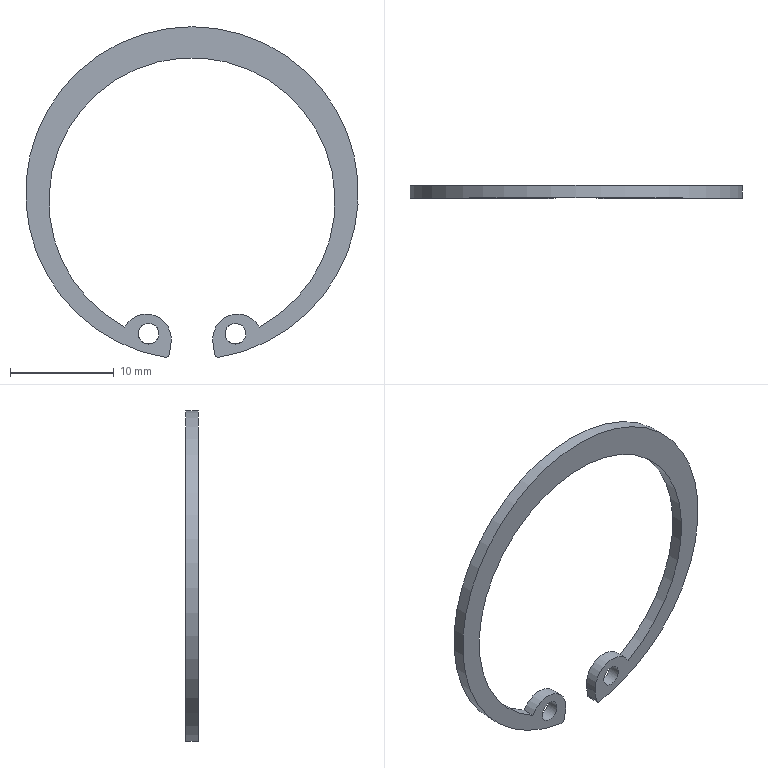Part | NX | features BREP 1 | 1 solid | 12 faces | box 32.1 x 1.2 x 31.887 mm | volume 256.127 mm3 | cylinder 8 | plane 4 | commonest cylinder face diameters 0.8 x2 2 x2 4.8 x2 27.6 x1 32.1 x1
STEP:
#1=CARTESIAN_POINT('',(-2.177,-1.2,-15.493));
#2=VERTEX_POINT('',#1);
#3=CARTESIAN_POINT('',(-2.639,-1.2,-15.832));
#4=VERTEX_POINT('',#3);
#5=CARTESIAN_POINT('',(-2.573,-1.2,-15.437));
#6=DIRECTION('',(0.,1.,0.));
#7=DIRECTION('',(0.,0.,1.));
#8=AXIS2_PLACEMENT_3D('',#5,#6,#7);
#9=CIRCLE('',#8,0.4);
#10=EDGE_CURVE('',#2,#4,#9,.T.);
#11=ORIENTED_EDGE('',*,*,#10,.T.);
#12=CARTESIAN_POINT('',(-2.639,0.,-15.832));
#13=VERTEX_POINT('',#12);
#14=CARTESIAN_POINT('',(-2.639,-1.2,-15.832));
#15=DIRECTION('',(0.,1.,0.));
#16=VECTOR('',#15,1000.);
#17=LINE('',#14,#16);
#18=EDGE_CURVE('',#4,#13,#17,.T.);
#19=ORIENTED_EDGE('',*,*,#18,.T.);
#20=CARTESIAN_POINT('',(-2.177,0.,-15.493));
#21=VERTEX_POINT('',#20);
#22=CARTESIAN_POINT('',(-2.573,0.,-15.437));
#23=DIRECTION('',(0.,1.,0.));
#24=DIRECTION('',(0.,0.,1.));
#25=AXIS2_PLACEMENT_3D('',#22,#23,#24);
#26=CIRCLE('',#25,0.4);
#27=EDGE_CURVE('',#21,#13,#26,.T.);
#28=ORIENTED_EDGE('',*,*,#27,.F.);
#29=CARTESIAN_POINT('',(-2.177,-1.2,-15.493));
#30=DIRECTION('',(0.,1.,0.));
#31=VECTOR('',#30,1000.);
#32=LINE('',#29,#31);
#33=EDGE_CURVE('',#2,#21,#32,.T.);
#34=ORIENTED_EDGE('',*,*,#33,.F.);
#35=EDGE_LOOP('',(#11,#19,#28,#34));
#36=FACE_BOUND('',#35,.T.);
#37=CARTESIAN_POINT('',(-2.573,-1.2,-15.437));
#38=DIRECTION('',(0.,1.,0.));
#39=DIRECTION('',(0.,0.,1.));
#40=AXIS2_PLACEMENT_3D('',#37,#38,#39);
#41=CYLINDRICAL_SURFACE('',#40,0.4);
#42=ADVANCED_FACE('',(#36),#41,.T.);
#43=CARTESIAN_POINT('',(2.639,-1.2,-15.832));
#44=VERTEX_POINT('',#43);
#45=CARTESIAN_POINT('',(2.177,-1.2,-15.493));
#46=VERTEX_POINT('',#45);
#47=CARTESIAN_POINT('',(2.573,-1.2,-15.437));
#48=DIRECTION('',(0.,1.,0.));
#49=DIRECTION('',(0.,0.,1.));
#50=AXIS2_PLACEMENT_3D('',#47,#48,#49);
#51=CIRCLE('',#50,0.4);
#52=EDGE_CURVE('',#44,#46,#51,.T.);
#53=ORIENTED_EDGE('',*,*,#52,.T.);
#54=CARTESIAN_POINT('',(2.177,0.,-15.493));
#55=VERTEX_POINT('',#54);
#56=CARTESIAN_POINT('',(2.177,-1.2,-15.493));
#57=DIRECTION('',(0.,1.,0.));
#58=VECTOR('',#57,1000.);
#59=LINE('',#56,#58);
#60=EDGE_CURVE('',#46,#55,#59,.T.);
#61=ORIENTED_EDGE('',*,*,#60,.T.);
#62=CARTESIAN_POINT('',(2.639,0.,-15.832));
#63=VERTEX_POINT('',#62);
#64=CARTESIAN_POINT('',(2.573,0.,-15.437));
#65=DIRECTION('',(0.,1.,0.));
#66=DIRECTION('',(0.,0.,1.));
#67=AXIS2_PLACEMENT_3D('',#64,#65,#66);
#68=CIRCLE('',#67,0.4);
#69=EDGE_CURVE('',#63,#55,#68,.T.);
#70=ORIENTED_EDGE('',*,*,#69,.F.);
#71=CARTESIAN_POINT('',(2.639,-1.2,-15.832));
#72=DIRECTION('',(0.,1.,0.));
#73=VECTOR('',#72,1000.);
#74=LINE('',#71,#73);
#75=EDGE_CURVE('',#44,#63,#74,.T.);
#76=ORIENTED_EDGE('',*,*,#75,.F.);
#77=EDGE_LOOP('',(#53,#61,#70,#76));
#78=FACE_BOUND('',#77,.T.);
#79=CARTESIAN_POINT('',(2.573,-1.2,-15.437));
#80=DIRECTION('',(0.,1.,0.));
#81=DIRECTION('',(0.,0.,1.));
#82=AXIS2_PLACEMENT_3D('',#79,#80,#81);
#83=CYLINDRICAL_SURFACE('',#82,0.4);
#84=ADVANCED_FACE('',(#78),#83,.T.);
#85=CARTESIAN_POINT('',(5.192,0.,-13.566));
#86=VERTEX_POINT('',#85);
#87=CARTESIAN_POINT('',(4.192,0.,-13.566));
#88=DIRECTION('',(0.,1.,0.));
#89=DIRECTION('',(1.,0.,0.));
#90=AXIS2_PLACEMENT_3D('',#87,#88,#89);
#91=CIRCLE('',#90,1.);
#92=EDGE_CURVE('',#86,#86,#91,.T.);
#93=ORIENTED_EDGE('',*,*,#92,.T.);
#94=EDGE_LOOP('',(#93));
#95=FACE_BOUND('',#94,.T.);
#96=CARTESIAN_POINT('',(4.192,-1.2,-12.566));
#97=VERTEX_POINT('',#96);
#98=CARTESIAN_POINT('',(4.192,-1.2,-13.566));
#99=DIRECTION('',(0.,1.,0.));
#100=DIRECTION('',(0.,0.,1.));
#101=AXIS2_PLACEMENT_3D('',#98,#99,#100);
#102=CIRCLE('',#101,1.);
#103=EDGE_CURVE('',#97,#97,#102,.T.);
#104=ORIENTED_EDGE('',*,*,#103,.F.);
#105=EDGE_LOOP('',(#104));
#106=FACE_BOUND('',#105,.T.);
#107=CARTESIAN_POINT('',(4.192,-45.302,-13.566));
#108=DIRECTION('',(0.,1.,0.));
#109=DIRECTION('',(0.,0.,1.));
#110=AXIS2_PLACEMENT_3D('',#107,#108,#109);
#111=CYLINDRICAL_SURFACE('',#110,1.);
#112=ADVANCED_FACE('',(#95,#106),#111,.F.);
#113=CARTESIAN_POINT('',(-3.192,0.,-13.566));
#114=VERTEX_POINT('',#113);
#115=CARTESIAN_POINT('',(-4.192,0.,-13.566));
#116=DIRECTION('',(0.,1.,0.));
#117=DIRECTION('',(1.,0.,0.));
#118=AXIS2_PLACEMENT_3D('',#115,#116,#117);
#119=CIRCLE('',#118,1.);
#120=EDGE_CURVE('',#114,#114,#119,.T.);
#121=ORIENTED_EDGE('',*,*,#120,.T.);
#122=EDGE_LOOP('',(#121));
#123=FACE_BOUND('',#122,.T.);
#124=CARTESIAN_POINT('',(-4.192,-1.2,-12.566));
#125=VERTEX_POINT('',#124);
#126=CARTESIAN_POINT('',(-4.192,-1.2,-13.566));
#127=DIRECTION('',(0.,1.,0.));
#128=DIRECTION('',(0.,0.,1.));
#129=AXIS2_PLACEMENT_3D('',#126,#127,#128);
#130=CIRCLE('',#129,1.);
#131=EDGE_CURVE('',#125,#125,#130,.T.);
#132=ORIENTED_EDGE('',*,*,#131,.F.);
#133=EDGE_LOOP('',(#132));
#134=FACE_BOUND('',#133,.T.);
#135=CARTESIAN_POINT('',(-4.192,-45.302,-13.566));
#136=DIRECTION('',(0.,1.,0.));
#137=DIRECTION('',(0.,0.,1.));
#138=AXIS2_PLACEMENT_3D('',#135,#136,#137);
#139=CYLINDRICAL_SURFACE('',#138,1.);
#140=ADVANCED_FACE('',(#123,#134),#139,.F.);
#141=CARTESIAN_POINT('',(-2.025,0.,-14.408));
#142=VERTEX_POINT('',#141);
#143=CARTESIAN_POINT('',(-2.234,0.,-15.894));
#144=DIRECTION('',(-0.1392,0.,-0.9903));
#145=VECTOR('',#144,1000.);
#146=LINE('',#143,#145);
#147=EDGE_CURVE('',#142,#21,#146,.T.);
#148=ORIENTED_EDGE('',*,*,#147,.T.);
#149=ORIENTED_EDGE('',*,*,#27,.T.);
#150=CARTESIAN_POINT('',(0.,0.,0.));
#151=DIRECTION('',(0.,1.,0.));
#152=DIRECTION('',(0.,0.,-1.));
#153=AXIS2_PLACEMENT_3D('',#150,#151,#152);
#154=CIRCLE('',#153,16.05);
#155=EDGE_CURVE('',#13,#63,#154,.T.);
#156=ORIENTED_EDGE('',*,*,#155,.T.);
#157=ORIENTED_EDGE('',*,*,#69,.T.);
#158=CARTESIAN_POINT('',(2.025,0.,-14.408));
#159=VERTEX_POINT('',#158);
#160=CARTESIAN_POINT('',(2.234,0.,-15.894));
#161=DIRECTION('',(-0.1392,0.,0.9903));
#162=VECTOR('',#161,1000.);
#163=LINE('',#160,#162);
#164=EDGE_CURVE('',#55,#159,#163,.T.);
#165=ORIENTED_EDGE('',*,*,#164,.T.);
#166=CARTESIAN_POINT('',(6.506,0.,-12.92));
#167=VERTEX_POINT('',#166);
#168=CARTESIAN_POINT('',(4.402,0.,-14.074));
#169=DIRECTION('',(0.,1.,0.));
#170=DIRECTION('',(1.,0.,0.));
#171=AXIS2_PLACEMENT_3D('',#168,#169,#170);
#172=CIRCLE('',#171,2.4);
#173=EDGE_CURVE('',#159,#167,#172,.T.);
#174=ORIENTED_EDGE('',*,*,#173,.T.);
#175=CARTESIAN_POINT('',(-6.506,0.,-12.92));
#176=VERTEX_POINT('',#175);
#177=CARTESIAN_POINT('',(0.,0.,-0.75));
#178=DIRECTION('',(0.,-1.,0.));
#179=DIRECTION('',(0.,0.,-1.));
#180=AXIS2_PLACEMENT_3D('',#177,#178,#179);
#181=CIRCLE('',#180,13.8);
#182=EDGE_CURVE('',#167,#176,#181,.T.);
#183=ORIENTED_EDGE('',*,*,#182,.T.);
#184=CARTESIAN_POINT('',(-4.402,0.,-14.074));
#185=DIRECTION('',(0.,1.,0.));
#186=DIRECTION('',(-1.,0.,0.));
#187=AXIS2_PLACEMENT_3D('',#184,#185,#186);
#188=CIRCLE('',#187,2.4);
#189=EDGE_CURVE('',#176,#142,#188,.T.);
#190=ORIENTED_EDGE('',*,*,#189,.T.);
#191=EDGE_LOOP('',(#148,#149,#156,#157,#165,#174,#183,#190));
#192=FACE_BOUND('',#191,.T.);
#193=ORIENTED_EDGE('',*,*,#120,.F.);
#194=EDGE_LOOP('',(#193));
#195=FACE_BOUND('',#194,.T.);
#196=ORIENTED_EDGE('',*,*,#92,.F.);
#197=EDGE_LOOP('',(#196));
#198=FACE_BOUND('',#197,.T.);
#199=CARTESIAN_POINT('',(0.,0.,0.));
#200=DIRECTION('',(0.,1.,0.));
#201=DIRECTION('',(0.,0.,1.));
#202=AXIS2_PLACEMENT_3D('',#199,#200,#201);
#203=PLANE('',#202);
#204=ADVANCED_FACE('',(#192,#195,#198),#203,.T.);
#205=CARTESIAN_POINT('',(0.,-1.2,0.));
#206=DIRECTION('',(0.,1.,0.));
#207=DIRECTION('',(0.,0.,-1.));
#208=AXIS2_PLACEMENT_3D('',#205,#206,#207);
#209=CIRCLE('',#208,16.05);
#210=EDGE_CURVE('',#4,#44,#209,.T.);
#211=ORIENTED_EDGE('',*,*,#210,.F.);
#212=ORIENTED_EDGE('',*,*,#10,.F.);
#213=CARTESIAN_POINT('',(-2.025,-1.2,-14.408));
#214=VERTEX_POINT('',#213);
#215=CARTESIAN_POINT('',(-2.234,-1.2,-15.894));
#216=DIRECTION('',(-0.1392,0.,-0.9903));
#217=VECTOR('',#216,1000.);
#218=LINE('',#215,#217);
#219=EDGE_CURVE('',#214,#2,#218,.T.);
#220=ORIENTED_EDGE('',*,*,#219,.F.);
#221=CARTESIAN_POINT('',(-6.506,-1.2,-12.92));
#222=VERTEX_POINT('',#221);
#223=CARTESIAN_POINT('',(-4.402,-1.2,-14.074));
#224=DIRECTION('',(0.,1.,0.));
#225=DIRECTION('',(-1.,0.,0.));
#226=AXIS2_PLACEMENT_3D('',#223,#224,#225);
#227=CIRCLE('',#226,2.4);
#228=EDGE_CURVE('',#222,#214,#227,.T.);
#229=ORIENTED_EDGE('',*,*,#228,.F.);
#230=CARTESIAN_POINT('',(6.506,-1.2,-12.92));
#231=VERTEX_POINT('',#230);
#232=CARTESIAN_POINT('',(0.,-1.2,-0.75));
#233=DIRECTION('',(0.,-1.,0.));
#234=DIRECTION('',(0.,0.,-1.));
#235=AXIS2_PLACEMENT_3D('',#232,#233,#234);
#236=CIRCLE('',#235,13.8);
#237=EDGE_CURVE('',#231,#222,#236,.T.);
#238=ORIENTED_EDGE('',*,*,#237,.F.);
#239=CARTESIAN_POINT('',(2.025,-1.2,-14.408));
#240=VERTEX_POINT('',#239);
#241=CARTESIAN_POINT('',(4.402,-1.2,-14.074));
#242=DIRECTION('',(0.,1.,0.));
#243=DIRECTION('',(1.,0.,0.));
#244=AXIS2_PLACEMENT_3D('',#241,#242,#243);
#245=CIRCLE('',#244,2.4);
#246=EDGE_CURVE('',#240,#231,#245,.T.);
#247=ORIENTED_EDGE('',*,*,#246,.F.);
#248=CARTESIAN_POINT('',(2.234,-1.2,-15.894));
#249=DIRECTION('',(-0.1392,0.,0.9903));
#250=VECTOR('',#249,1000.);
#251=LINE('',#248,#250);
#252=EDGE_CURVE('',#46,#240,#251,.T.);
#253=ORIENTED_EDGE('',*,*,#252,.F.);
#254=ORIENTED_EDGE('',*,*,#52,.F.);
#255=EDGE_LOOP('',(#211,#212,#220,#229,#238,#247,#253,#254));
#256=FACE_BOUND('',#255,.T.);
#257=ORIENTED_EDGE('',*,*,#131,.T.);
#258=EDGE_LOOP('',(#257));
#259=FACE_BOUND('',#258,.T.);
#260=ORIENTED_EDGE('',*,*,#103,.T.);
#261=EDGE_LOOP('',(#260));
#262=FACE_BOUND('',#261,.T.);
#263=CARTESIAN_POINT('',(0.,-1.2,0.));
#264=DIRECTION('',(0.,1.,0.));
#265=DIRECTION('',(0.,0.,1.));
#266=AXIS2_PLACEMENT_3D('',#263,#264,#265);
#267=PLANE('',#266);
#268=ADVANCED_FACE('',(#256,#259,#262),#267,.F.);
#269=ORIENTED_EDGE('',*,*,#189,.F.);
#270=CARTESIAN_POINT('',(-6.506,-1.2,-12.92));
#271=DIRECTION('',(0.,1.,0.));
#272=VECTOR('',#271,1000.);
#273=LINE('',#270,#272);
#274=EDGE_CURVE('',#222,#176,#273,.T.);
#275=ORIENTED_EDGE('',*,*,#274,.F.);
#276=ORIENTED_EDGE('',*,*,#228,.T.);
#277=CARTESIAN_POINT('',(-2.025,-1.2,-14.408));
#278=DIRECTION('',(0.,1.,0.));
#279=VECTOR('',#278,1000.);
#280=LINE('',#277,#279);
#281=EDGE_CURVE('',#214,#142,#280,.T.);
#282=ORIENTED_EDGE('',*,*,#281,.T.);
#283=EDGE_LOOP('',(#269,#275,#276,#282));
#284=FACE_BOUND('',#283,.T.);
#285=CARTESIAN_POINT('',(-4.402,-1.2,-14.074));
#286=DIRECTION('',(0.,1.,0.));
#287=DIRECTION('',(0.,0.,1.));
#288=AXIS2_PLACEMENT_3D('',#285,#286,#287);
#289=CYLINDRICAL_SURFACE('',#288,2.4);
#290=ADVANCED_FACE('',(#284),#289,.T.);
#291=ORIENTED_EDGE('',*,*,#182,.F.);
#292=CARTESIAN_POINT('',(6.506,-1.2,-12.92));
#293=DIRECTION('',(0.,1.,0.));
#294=VECTOR('',#293,1000.);
#295=LINE('',#292,#294);
#296=EDGE_CURVE('',#231,#167,#295,.T.);
#297=ORIENTED_EDGE('',*,*,#296,.F.);
#298=ORIENTED_EDGE('',*,*,#237,.T.);
#299=ORIENTED_EDGE('',*,*,#274,.T.);
#300=EDGE_LOOP('',(#291,#297,#298,#299));
#301=FACE_BOUND('',#300,.T.);
#302=CARTESIAN_POINT('',(0.,-1.2,-0.75));
#303=DIRECTION('',(0.,1.,0.));
#304=DIRECTION('',(0.,0.,1.));
#305=AXIS2_PLACEMENT_3D('',#302,#303,#304);
#306=CYLINDRICAL_SURFACE('',#305,13.8);
#307=ADVANCED_FACE('',(#301),#306,.F.);
#308=ORIENTED_EDGE('',*,*,#173,.F.);
#309=CARTESIAN_POINT('',(2.025,-1.2,-14.408));
#310=DIRECTION('',(0.,1.,0.));
#311=VECTOR('',#310,1000.);
#312=LINE('',#309,#311);
#313=EDGE_CURVE('',#240,#159,#312,.T.);
#314=ORIENTED_EDGE('',*,*,#313,.F.);
#315=ORIENTED_EDGE('',*,*,#246,.T.);
#316=ORIENTED_EDGE('',*,*,#296,.T.);
#317=EDGE_LOOP('',(#308,#314,#315,#316));
#318=FACE_BOUND('',#317,.T.);
#319=CARTESIAN_POINT('',(4.402,-1.2,-14.074));
#320=DIRECTION('',(0.,1.,0.));
#321=DIRECTION('',(0.,0.,1.));
#322=AXIS2_PLACEMENT_3D('',#319,#320,#321);
#323=CYLINDRICAL_SURFACE('',#322,2.4);
#324=ADVANCED_FACE('',(#318),#323,.T.);
#325=ORIENTED_EDGE('',*,*,#164,.F.);
#326=ORIENTED_EDGE('',*,*,#60,.F.);
#327=ORIENTED_EDGE('',*,*,#252,.T.);
#328=ORIENTED_EDGE('',*,*,#313,.T.);
#329=EDGE_LOOP('',(#325,#326,#327,#328));
#330=FACE_BOUND('',#329,.T.);
#331=CARTESIAN_POINT('',(2.234,-1.2,-15.894));
#332=DIRECTION('',(-0.9903,0.,-0.1392));
#333=DIRECTION('',(-0.1392,0.,0.9903));
#334=AXIS2_PLACEMENT_3D('',#331,#332,#333);
#335=PLANE('',#334);
#336=ADVANCED_FACE('',(#330),#335,.T.);
#337=ORIENTED_EDGE('',*,*,#155,.F.);
#338=ORIENTED_EDGE('',*,*,#18,.F.);
#339=ORIENTED_EDGE('',*,*,#210,.T.);
#340=ORIENTED_EDGE('',*,*,#75,.T.);
#341=EDGE_LOOP('',(#337,#338,#339,#340));
#342=FACE_BOUND('',#341,.T.);
#343=CARTESIAN_POINT('',(0.,-1.2,0.));
#344=DIRECTION('',(0.,1.,0.));
#345=DIRECTION('',(0.,0.,1.));
#346=AXIS2_PLACEMENT_3D('',#343,#344,#345);
#347=CYLINDRICAL_SURFACE('',#346,16.05);
#348=ADVANCED_FACE('',(#342),#347,.T.);
#349=ORIENTED_EDGE('',*,*,#219,.T.);
#350=ORIENTED_EDGE('',*,*,#33,.T.);
#351=ORIENTED_EDGE('',*,*,#147,.F.);
#352=ORIENTED_EDGE('',*,*,#281,.F.);
#353=EDGE_LOOP('',(#349,#350,#351,#352));
#354=FACE_BOUND('',#353,.T.);
#355=CARTESIAN_POINT('',(-2.234,-1.2,-15.894));
#356=DIRECTION('',(0.9903,0.,-0.1392));
#357=DIRECTION('',(-0.1392,0.,-0.9903));
#358=AXIS2_PLACEMENT_3D('',#355,#356,#357);
#359=PLANE('',#358);
#360=ADVANCED_FACE('',(#354),#359,.T.);
#361=CLOSED_SHELL('',(#42,#84,#112,#140,#204,#268,#290,#307,#324,#336,#348,#360));
#362=MANIFOLD_SOLID_BREP('',#361);
#363=(LENGTH_UNIT()NAMED_UNIT(*)SI_UNIT(.MILLI.,.METRE.));
#364=UNCERTAINTY_MEASURE_WITH_UNIT(LENGTH_MEASURE(0.00001),#363,'','');
#365=(NAMED_UNIT(*)PLANE_ANGLE_UNIT()SI_UNIT($,.RADIAN.));
#366=(NAMED_UNIT(*)SI_UNIT($,.STERADIAN.)SOLID_ANGLE_UNIT());
#367=(GEOMETRIC_REPRESENTATION_CONTEXT(3)GLOBAL_UNCERTAINTY_ASSIGNED_CONTEXT((#364))GLOBAL_UNIT_ASSIGNED_CONTEXT((#363,#365,#366))REPRESENTATION_CONTEXT('',''));
#368=ADVANCED_BREP_SHAPE_REPRESENTATION('',(#362),#367);